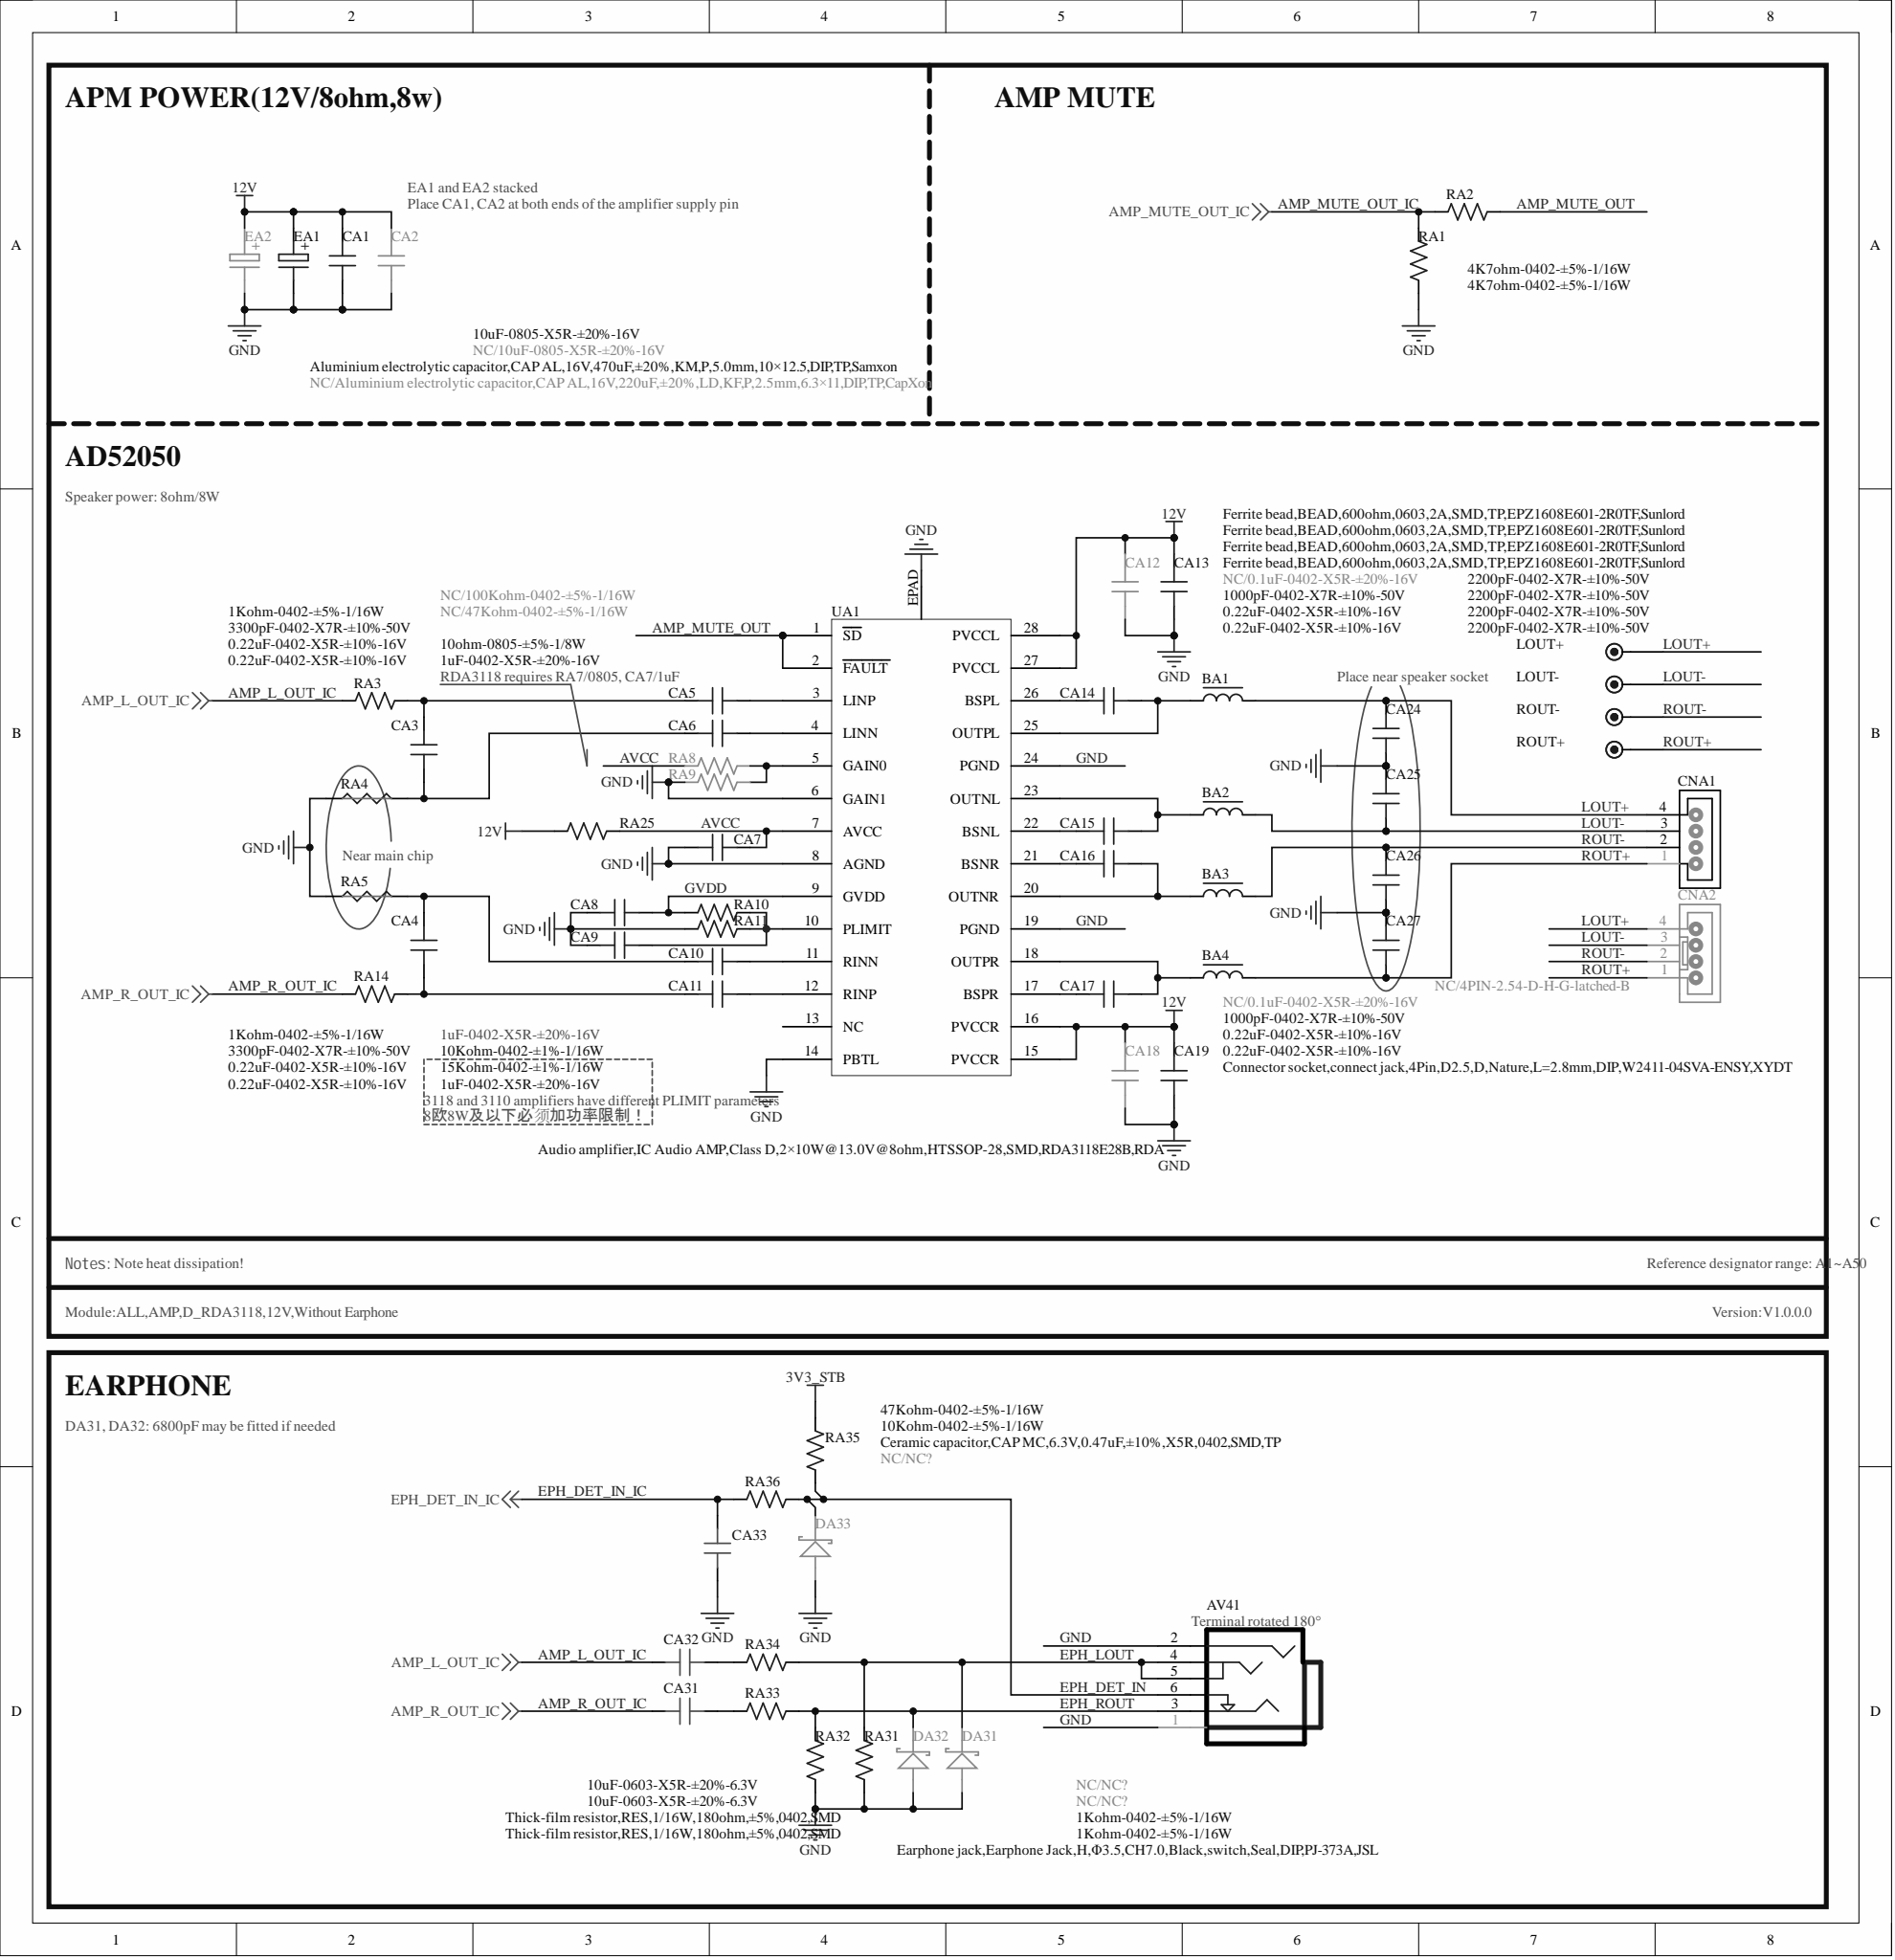Circuit board | Altium Designer | 578 parts | 300 nets | one sheet of the schematic
Parts on this sheet (reference | value | footprint):
AV41 | Earphone jack,Earphone Jack,H,F3.5,CH7.0,Black,switch,Seal,DIP,PJ-373A,JSL | PHONE-HD-42
BA1 | Ferrite bead,BEAD,600ohm,0603,2A,SMD,TP,EPZ1608E601-2R0TF,Sunlord | L0603
BA2 | Ferrite bead,BEAD,600ohm,0603,2A,SMD,TP,EPZ1608E601-2R0TF,Sunlord | L0603
BA3 | Ferrite bead,BEAD,600ohm,0603,2A,SMD,TP,EPZ1608E601-2R0TF,Sunlord | L0603
BA4 | Ferrite bead,BEAD,600ohm,0603,2A,SMD,TP,EPZ1608E601-2R0TF,Sunlord | L0603
CA1 | 10uF-0805-X5R-±20%-16V | C0805
CA2 | NC/10uF-0805-X5R-±20%-16V | C0805
CA3 | 3300pF-0402-X7R-±10%-50V | C0402
CA4 | 3300pF-0402-X7R-±10%-50V | C0402
CA5 | 0.22uF-0402-X5R-±10%-16V | C0402
CA6 | 0.22uF-0402-X5R-±10%-16V | C0402
CA7 | 1uF-0402-X5R-±20%-16V | C0402
CA8 | 1uF-0402-X5R-±20%-16V | C0402
CA9 | 1uF-0402-X5R-±20%-16V | C0402
CA10 | 0.22uF-0402-X5R-±10%-16V | C0402
CA11 | 0.22uF-0402-X5R-±10%-16V | C0402
CA12 | NC/0.1uF-0402-X5R-±20%-16V | C0402
CA13 | 1000pF-0402-X7R-±10%-50V | C0402
CA14 | 0.22uF-0402-X5R-±10%-16V | C0402
CA15 | 0.22uF-0402-X5R-±10%-16V | C0402
CA16 | 0.22uF-0402-X5R-±10%-16V | C0402
CA17 | 0.22uF-0402-X5R-±10%-16V | C0402
CA18 | NC/0.1uF-0402-X5R-±20%-16V | C0402
CA19 | 1000pF-0402-X7R-±10%-50V | C0402
CA24 | 2200pF-0402-X7R-±10%-50V | C0402
CA25 | 2200pF-0402-X7R-±10%-50V | C0402
CA26 | 2200pF-0402-X7R-±10%-50V | C0402
CA27 | 2200pF-0402-X7R-±10%-50V | C0402
CA31 | 10uF-0603-X5R-±20%-6.3V | C0603
CA32 | 10uF-0603-X5R-±20%-6.3V | C0603
CA33 | Ceramic capacitor,CAP MC,6.3V,0.47uF,±10%,X5R,0402,SMD,TP | C0402
CNA1 | Connector socket,connect jack,4Pin,D2.5,D,Nature,L=2.8mm,DIP,W2411-04SVA-ENSY,XYDT | SIP4/2.54D-1
CNA2 | NC/4PIN-2.54-D-H-G-latched-B | SIP4/2.5D-2
DA31 | NC/NC? | DIODE-S0402
DA32 | NC/NC? | DIODE-S0402
DA33 | NC/NC? | DIODE-S0402
EA1 | Aluminium electrolytic capacitor,CAP AL,16V,470uF,±20%,KM,P,5.0mm,10×12.5,DIP,TP,Samxon | EC(10*12)-V-5
EA2 | NC/Aluminium electrolytic capacitor,CAP AL,16V,220uF,±20%,LD,KF,P,2.5mm,6.3×11,DIP,TP,CapXon | EC(6.3*11)-V-2.5
LOUT+ | DM0 | TP
LOUT- | DM0 | TP
RA1 | 4K7ohm-0402-±5%-1/16W | R0402
RA2 | 4K7ohm-0402-±5%-1/16W | R0402
RA3 | 1Kohm-0402-±5%-1/16W | R0402
RA4 | NC/? | GND
RA5 | NC/? | GND
RA8 | NC/100Kohm-0402-±5%-1/16W | R0402
RA9 | NC/47Kohm-0402-±5%-1/16W | R0402
RA10 | 10Kohm-0402-±1%-1/16W | R0402
RA11 | 15Kohm-0402-±1%-1/16W | R0402
RA14 | 1Kohm-0402-±5%-1/16W | R0402
RA25 | 10ohm-0805-±5%-1/8W | R0805
RA31 | 1Kohm-0402-±5%-1/16W | R0402
RA32 | 1Kohm-0402-±5%-1/16W | R0402
RA33 | Thick-film resistor,RES,1/16W,180ohm,±5%,0402,SMD | R0402
RA34 | Thick-film resistor,RES,1/16W,180ohm,±5%,0402,SMD | R0402
RA35 | 47Kohm-0402-±5%-1/16W | R0402
RA36 | 10Kohm-0402-±5%-1/16W | R0402
ROUT+ | DM0 | TP
UA1 | Audio amplifier,IC Audio AMP,Class D,2×10W@13.0V@8ohm,HTSSOP-28,SMD,RDA3118E28B,RDA | SSOP28/0.65-5
Nets of these parts (net: part-pin ...):
ROUT-: BA3-2 CA26-2 CNA1-2 CNA2-2
ROUT+: BA4-2 CA27-1 CNA1-1 CNA2-1 ROUT+-1
NetRA8_2: RA8-2 RA9-2 UA1-5
NetCA32_1: CA32-1 RA34-1
NetCA31_1: CA31-1 RA33-1
NetCA17_1: CA17-1 UA1-17
NetCA16_1: CA16-1 UA1-21
NetCA15_1: CA15-1 UA1-22
NetCA14_1: CA14-1 UA1-26
NetCA11_2: CA11-2 UA1-12
NetCA10_2: CA10-2 UA1-11
NetCA9_2: CA9-2 RA10-2 RA11-2 UA1-10
NetCA6_2: CA6-2 UA1-4
NetCA5_2: CA5-2 UA1-3
NetCA4_2: CA4-2 CA10-1 RA5-JP_1K
NetCA4_1: CA4-1 CA11-1 RA14-2
NetCA3_2: CA3-2 CA5-1 RA3-2
NetCA3_1: CA3-1 CA6-1 RA4-JP_1K
NetBA4_1: BA4-1 CA17-2 UA1-18
NetBA3_1: BA3-1 CA16-2 UA1-20
NetBA2_1: BA2-1 CA15-2 UA1-23
NetBA1_1: BA1-1 CA14-2 UA1-25
LOUT-: BA2-2 CA25-1 CNA1-3 CNA2-3 LOUT--1
LOUT+: BA1-2 CA24-2 CNA1-4 CNA2-4 LOUT+-1
GVDD: CA8-2 RA10-1 UA1-9
GND: AV41-1 AV41-2 CA1-1 CA2-1 CA7-1 CA8-1 CA9-1 CA12-1 CA13-1 CA18-1 CA19-1 CA24-1 CA25-2 CA26-1 CA27-2 CA33-1 DA31-A DA32-A DA33-A EA1-2 EA2-2 RA1-2 RA4-JP_2K RA5-JP_2K RA9-1 RA11-1 RA31-1 RA32-1 UA1-6 UA1-8 UA1-14 UA1-19 UA1-24 UA1-EPAD
EPH_ROUT: AV41-3 DA32-K RA32-2 RA33-2
EPH_LOUT: AV41-4 AV41-5 DA31-K RA31-2 RA34-2
EPH_DET_IN_IC: CA33-2 RA36-1
EPH_DET_IN: AV41-6 DA33-K RA35-1 RA36-2
AVCC: CA7-2 RA8-1 RA25-2 UA1-7
AMP_R_OUT_IC: CA31-2 RA14-1
AMP_MUTE_OUT_IC: RA1-1 RA2-2
AMP_MUTE_OUT: RA2-1 UA1-1 UA1-2
AMP_L_OUT_IC: CA32-2 RA3-1
12V: CA1-2 CA2-2 CA12-2 CA13-2 CA18-2 CA19-2 EA1-1 EA2-1 RA25-1 UA1-15 UA1-16 UA1-27 UA1-28
3V3_STB: RA35-2